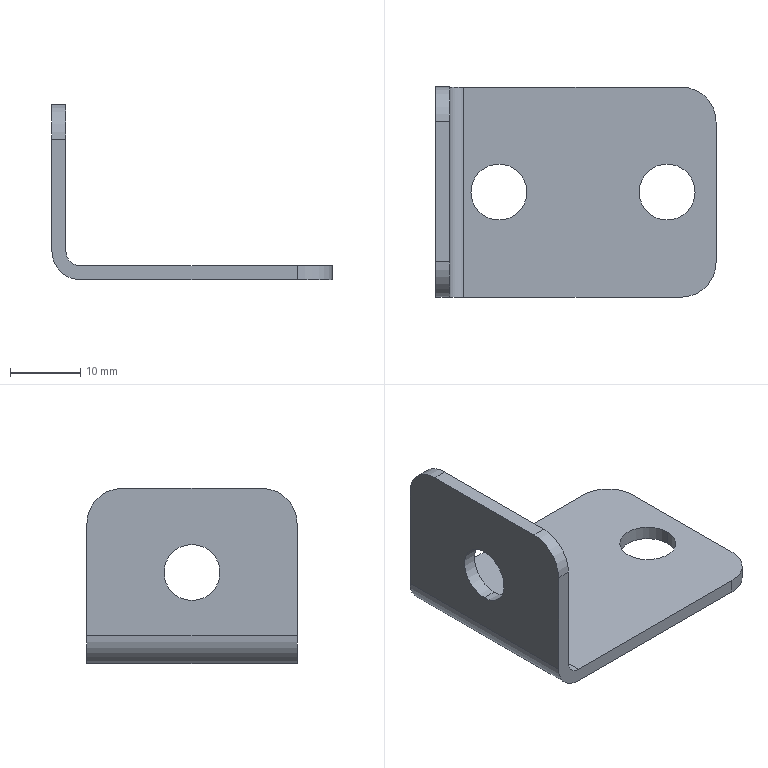Part | STEP file | 921271505 | 1 solid | 20 faces | box 40 x 30 x 25 mm | volume 3358 mm3 | cylinder 12 | plane 8 | commonest cylinder face diameters 8 x7 10 x4 4 x1
STEP:
#1=CARTESIAN_POINT('',(5.,15.,2.));
#2=VERTEX_POINT('',#1);
#3=CARTESIAN_POINT('',(13.,15.,2.));
#4=VERTEX_POINT('',#3);
#5=CARTESIAN_POINT('',(9.,15.,2.));
#6=DIRECTION('',(0.,0.,1.));
#7=DIRECTION('',(-1.,0.,0.));
#8=AXIS2_PLACEMENT_3D('',#5,#6,#7);
#9=CIRCLE('',#8,4.);
#10=EDGE_CURVE('',#2,#4,#9,.T.);
#11=ORIENTED_EDGE('',*,*,#10,.T.);
#12=CARTESIAN_POINT('',(13.,15.,0.));
#13=VERTEX_POINT('',#12);
#14=CARTESIAN_POINT('',(13.,15.,55.902));
#15=DIRECTION('',(0.,0.,-1.));
#16=VECTOR('',#15,1000.);
#17=LINE('',#14,#16);
#18=EDGE_CURVE('',#4,#13,#17,.T.);
#19=ORIENTED_EDGE('',*,*,#18,.T.);
#20=CARTESIAN_POINT('',(5.,15.,0.));
#21=VERTEX_POINT('',#20);
#22=CARTESIAN_POINT('',(9.,15.,0.));
#23=DIRECTION('',(0.,0.,1.));
#24=DIRECTION('',(-1.,0.,0.));
#25=AXIS2_PLACEMENT_3D('',#22,#23,#24);
#26=CIRCLE('',#25,4.);
#27=EDGE_CURVE('',#21,#13,#26,.T.);
#28=ORIENTED_EDGE('',*,*,#27,.F.);
#29=CARTESIAN_POINT('',(5.,15.,55.902));
#30=DIRECTION('',(0.,0.,-1.));
#31=VECTOR('',#30,1000.);
#32=LINE('',#29,#31);
#33=EDGE_CURVE('',#2,#21,#32,.T.);
#34=ORIENTED_EDGE('',*,*,#33,.F.);
#35=EDGE_LOOP('',(#11,#19,#28,#34));
#36=FACE_OUTER_BOUND('',#35,.T.);
#37=CARTESIAN_POINT('',(9.,15.,55.902));
#38=DIRECTION('',(0.,0.,-1.));
#39=DIRECTION('',(-1.,0.,0.));
#40=AXIS2_PLACEMENT_3D('',#37,#38,#39);
#41=CYLINDRICAL_SURFACE('',#40,4.);
#42=ADVANCED_FACE('',(#36),#41,.F.);
#43=CARTESIAN_POINT('',(29.,15.,2.));
#44=VERTEX_POINT('',#43);
#45=CARTESIAN_POINT('',(37.,15.,2.));
#46=VERTEX_POINT('',#45);
#47=CARTESIAN_POINT('',(33.,15.,2.));
#48=DIRECTION('',(0.,0.,1.));
#49=DIRECTION('',(-1.,0.,0.));
#50=AXIS2_PLACEMENT_3D('',#47,#48,#49);
#51=CIRCLE('',#50,4.);
#52=EDGE_CURVE('',#44,#46,#51,.T.);
#53=ORIENTED_EDGE('',*,*,#52,.T.);
#54=CARTESIAN_POINT('',(37.,15.,0.));
#55=VERTEX_POINT('',#54);
#56=CARTESIAN_POINT('',(37.,15.,55.902));
#57=DIRECTION('',(0.,0.,-1.));
#58=VECTOR('',#57,1000.);
#59=LINE('',#56,#58);
#60=EDGE_CURVE('',#46,#55,#59,.T.);
#61=ORIENTED_EDGE('',*,*,#60,.T.);
#62=CARTESIAN_POINT('',(29.,15.,0.));
#63=VERTEX_POINT('',#62);
#64=CARTESIAN_POINT('',(33.,15.,0.));
#65=DIRECTION('',(0.,0.,1.));
#66=DIRECTION('',(-1.,0.,0.));
#67=AXIS2_PLACEMENT_3D('',#64,#65,#66);
#68=CIRCLE('',#67,4.);
#69=EDGE_CURVE('',#63,#55,#68,.T.);
#70=ORIENTED_EDGE('',*,*,#69,.F.);
#71=CARTESIAN_POINT('',(29.,15.,55.902));
#72=DIRECTION('',(0.,0.,-1.));
#73=VECTOR('',#72,1000.);
#74=LINE('',#71,#73);
#75=EDGE_CURVE('',#44,#63,#74,.T.);
#76=ORIENTED_EDGE('',*,*,#75,.F.);
#77=EDGE_LOOP('',(#53,#61,#70,#76));
#78=FACE_OUTER_BOUND('',#77,.T.);
#79=CARTESIAN_POINT('',(33.,15.,55.902));
#80=DIRECTION('',(0.,0.,-1.));
#81=DIRECTION('',(-1.,0.,0.));
#82=AXIS2_PLACEMENT_3D('',#79,#80,#81);
#83=CYLINDRICAL_SURFACE('',#82,4.);
#84=ADVANCED_FACE('',(#78),#83,.F.);
#85=CARTESIAN_POINT('',(2.,15.,17.));
#86=VERTEX_POINT('',#85);
#87=CARTESIAN_POINT('',(2.,15.,9.));
#88=VERTEX_POINT('',#87);
#89=CARTESIAN_POINT('',(2.,15.,13.));
#90=DIRECTION('',(1.,0.,0.));
#91=DIRECTION('',(0.,0.,1.));
#92=AXIS2_PLACEMENT_3D('',#89,#90,#91);
#93=CIRCLE('',#92,4.);
#94=EDGE_CURVE('',#86,#88,#93,.T.);
#95=ORIENTED_EDGE('',*,*,#94,.T.);
#96=CARTESIAN_POINT('',(0.,15.,9.));
#97=VERTEX_POINT('',#96);
#98=CARTESIAN_POINT('',(55.902,15.,9.));
#99=DIRECTION('',(-1.,0.,0.));
#100=VECTOR('',#99,1000.);
#101=LINE('',#98,#100);
#102=EDGE_CURVE('',#88,#97,#101,.T.);
#103=ORIENTED_EDGE('',*,*,#102,.T.);
#104=CARTESIAN_POINT('',(0.,15.,17.));
#105=VERTEX_POINT('',#104);
#106=CARTESIAN_POINT('',(0.,15.,13.));
#107=DIRECTION('',(1.,0.,0.));
#108=DIRECTION('',(0.,0.,1.));
#109=AXIS2_PLACEMENT_3D('',#106,#107,#108);
#110=CIRCLE('',#109,4.);
#111=EDGE_CURVE('',#105,#97,#110,.T.);
#112=ORIENTED_EDGE('',*,*,#111,.F.);
#113=CARTESIAN_POINT('',(55.902,15.,17.));
#114=DIRECTION('',(-1.,0.,0.));
#115=VECTOR('',#114,1000.);
#116=LINE('',#113,#115);
#117=EDGE_CURVE('',#86,#105,#116,.T.);
#118=ORIENTED_EDGE('',*,*,#117,.F.);
#119=EDGE_LOOP('',(#95,#103,#112,#118));
#120=FACE_OUTER_BOUND('',#119,.T.);
#121=CARTESIAN_POINT('',(55.902,15.,13.));
#122=DIRECTION('',(-1.,0.,0.));
#123=DIRECTION('',(0.,0.,1.));
#124=AXIS2_PLACEMENT_3D('',#121,#122,#123);
#125=CYLINDRICAL_SURFACE('',#124,4.);
#126=ADVANCED_FACE('',(#120),#125,.F.);
#127=CARTESIAN_POINT('',(35.,30.,2.));
#128=VERTEX_POINT('',#127);
#129=CARTESIAN_POINT('',(40.,25.,2.));
#130=VERTEX_POINT('',#129);
#131=CARTESIAN_POINT('',(35.,25.,2.));
#132=DIRECTION('',(0.,0.,-1.));
#133=DIRECTION('',(-1.,0.,0.));
#134=AXIS2_PLACEMENT_3D('',#131,#132,#133);
#135=CIRCLE('',#134,5.);
#136=EDGE_CURVE('',#128,#130,#135,.T.);
#137=ORIENTED_EDGE('',*,*,#136,.F.);
#138=CARTESIAN_POINT('',(4.,30.,2.));
#139=VERTEX_POINT('',#138);
#140=CARTESIAN_POINT('',(0.,30.,2.));
#141=DIRECTION('',(1.,0.,0.));
#142=VECTOR('',#141,1000.);
#143=LINE('',#140,#142);
#144=EDGE_CURVE('',#139,#128,#143,.T.);
#145=ORIENTED_EDGE('',*,*,#144,.F.);
#146=CARTESIAN_POINT('',(4.,0.,2.));
#147=VERTEX_POINT('',#146);
#148=CARTESIAN_POINT('',(4.,0.,2.));
#149=DIRECTION('',(0.,1.,0.));
#150=VECTOR('',#149,1000.);
#151=LINE('',#148,#150);
#152=EDGE_CURVE('',#147,#139,#151,.T.);
#153=ORIENTED_EDGE('',*,*,#152,.F.);
#154=CARTESIAN_POINT('',(35.,0.,2.));
#155=VERTEX_POINT('',#154);
#156=CARTESIAN_POINT('',(0.,0.,2.));
#157=DIRECTION('',(-1.,0.,0.));
#158=VECTOR('',#157,1000.);
#159=LINE('',#156,#158);
#160=EDGE_CURVE('',#155,#147,#159,.T.);
#161=ORIENTED_EDGE('',*,*,#160,.F.);
#162=CARTESIAN_POINT('',(40.,5.,2.));
#163=VERTEX_POINT('',#162);
#164=CARTESIAN_POINT('',(35.,5.,2.));
#165=DIRECTION('',(0.,0.,-1.));
#166=DIRECTION('',(-1.,0.,0.));
#167=AXIS2_PLACEMENT_3D('',#164,#165,#166);
#168=CIRCLE('',#167,5.);
#169=EDGE_CURVE('',#163,#155,#168,.T.);
#170=ORIENTED_EDGE('',*,*,#169,.F.);
#171=CARTESIAN_POINT('',(40.,0.,2.));
#172=DIRECTION('',(0.,-1.,0.));
#173=VECTOR('',#172,1000.);
#174=LINE('',#171,#173);
#175=EDGE_CURVE('',#130,#163,#174,.T.);
#176=ORIENTED_EDGE('',*,*,#175,.F.);
#177=EDGE_LOOP('',(#137,#145,#153,#161,#170,#176));
#178=FACE_OUTER_BOUND('',#177,.T.);
#179=ORIENTED_EDGE('',*,*,#10,.F.);
#180=CARTESIAN_POINT('',(9.,15.,2.));
#181=DIRECTION('',(0.,0.,1.));
#182=DIRECTION('',(-1.,0.,0.));
#183=AXIS2_PLACEMENT_3D('',#180,#181,#182);
#184=CIRCLE('',#183,4.);
#185=EDGE_CURVE('',#4,#2,#184,.T.);
#186=ORIENTED_EDGE('',*,*,#185,.F.);
#187=EDGE_LOOP('',(#179,#186));
#188=FACE_BOUND('',#187,.T.);
#189=ORIENTED_EDGE('',*,*,#52,.F.);
#190=CARTESIAN_POINT('',(33.,15.,2.));
#191=DIRECTION('',(0.,0.,1.));
#192=DIRECTION('',(-1.,0.,0.));
#193=AXIS2_PLACEMENT_3D('',#190,#191,#192);
#194=CIRCLE('',#193,4.);
#195=EDGE_CURVE('',#46,#44,#194,.T.);
#196=ORIENTED_EDGE('',*,*,#195,.F.);
#197=EDGE_LOOP('',(#189,#196));
#198=FACE_BOUND('',#197,.T.);
#199=CARTESIAN_POINT('',(0.,0.,2.));
#200=DIRECTION('',(0.,0.,-1.));
#201=DIRECTION('',(-1.,0.,0.));
#202=AXIS2_PLACEMENT_3D('',#199,#200,#201);
#203=PLANE('',#202);
#204=ADVANCED_FACE('',(#178,#188,#198),#203,.F.);
#205=ORIENTED_EDGE('',*,*,#175,.T.);
#206=CARTESIAN_POINT('',(40.,5.,0.));
#207=VERTEX_POINT('',#206);
#208=CARTESIAN_POINT('',(40.,5.,2.));
#209=DIRECTION('',(0.,0.,-1.));
#210=VECTOR('',#209,1000.);
#211=LINE('',#208,#210);
#212=EDGE_CURVE('',#163,#207,#211,.T.);
#213=ORIENTED_EDGE('',*,*,#212,.T.);
#214=CARTESIAN_POINT('',(40.,25.,0.));
#215=VERTEX_POINT('',#214);
#216=CARTESIAN_POINT('',(40.,30.,0.));
#217=DIRECTION('',(0.,1.,0.));
#218=VECTOR('',#217,1000.);
#219=LINE('',#216,#218);
#220=EDGE_CURVE('',#207,#215,#219,.T.);
#221=ORIENTED_EDGE('',*,*,#220,.T.);
#222=CARTESIAN_POINT('',(40.,25.,2.));
#223=DIRECTION('',(0.,0.,1.));
#224=VECTOR('',#223,1000.);
#225=LINE('',#222,#224);
#226=EDGE_CURVE('',#215,#130,#225,.T.);
#227=ORIENTED_EDGE('',*,*,#226,.T.);
#228=EDGE_LOOP('',(#205,#213,#221,#227));
#229=FACE_OUTER_BOUND('',#228,.T.);
#230=CARTESIAN_POINT('',(40.,30.,2.));
#231=DIRECTION('',(1.,0.,0.));
#232=DIRECTION('',(0.,1.,0.));
#233=AXIS2_PLACEMENT_3D('',#230,#231,#232);
#234=PLANE('',#233);
#235=ADVANCED_FACE('',(#229),#234,.T.);
#236=CARTESIAN_POINT('',(35.,30.,0.));
#237=VERTEX_POINT('',#236);
#238=CARTESIAN_POINT('',(35.,25.,0.));
#239=DIRECTION('',(0.,0.,1.));
#240=DIRECTION('',(-1.,0.,0.));
#241=AXIS2_PLACEMENT_3D('',#238,#239,#240);
#242=CIRCLE('',#241,5.);
#243=EDGE_CURVE('',#215,#237,#242,.T.);
#244=ORIENTED_EDGE('',*,*,#243,.T.);
#245=CARTESIAN_POINT('',(35.,30.,2.));
#246=DIRECTION('',(0.,0.,1.));
#247=VECTOR('',#246,1000.);
#248=LINE('',#245,#247);
#249=EDGE_CURVE('',#237,#128,#248,.T.);
#250=ORIENTED_EDGE('',*,*,#249,.T.);
#251=ORIENTED_EDGE('',*,*,#136,.T.);
#252=ORIENTED_EDGE('',*,*,#226,.F.);
#253=EDGE_LOOP('',(#244,#250,#251,#252));
#254=FACE_OUTER_BOUND('',#253,.T.);
#255=CARTESIAN_POINT('',(35.,25.,2.));
#256=DIRECTION('',(0.,0.,-1.));
#257=DIRECTION('',(-1.,0.,0.));
#258=AXIS2_PLACEMENT_3D('',#255,#256,#257);
#259=CYLINDRICAL_SURFACE('',#258,5.);
#260=ADVANCED_FACE('',(#254),#259,.T.);
#261=CARTESIAN_POINT('',(4.,30.,0.));
#262=VERTEX_POINT('',#261);
#263=CARTESIAN_POINT('',(0.,30.,0.));
#264=DIRECTION('',(-1.,0.,0.));
#265=VECTOR('',#264,1000.);
#266=LINE('',#263,#265);
#267=EDGE_CURVE('',#237,#262,#266,.T.);
#268=ORIENTED_EDGE('',*,*,#267,.T.);
#269=CARTESIAN_POINT('',(0.,30.,4.));
#270=VERTEX_POINT('',#269);
#271=CARTESIAN_POINT('',(4.,30.,4.));
#272=DIRECTION('',(0.,1.,0.));
#273=DIRECTION('',(-1.,0.,0.));
#274=AXIS2_PLACEMENT_3D('',#271,#272,#273);
#275=CIRCLE('',#274,4.);
#276=EDGE_CURVE('',#262,#270,#275,.T.);
#277=ORIENTED_EDGE('',*,*,#276,.T.);
#278=CARTESIAN_POINT('',(0.,30.,20.));
#279=VERTEX_POINT('',#278);
#280=CARTESIAN_POINT('',(0.,30.,2.));
#281=DIRECTION('',(0.,0.,1.));
#282=VECTOR('',#281,1000.);
#283=LINE('',#280,#282);
#284=EDGE_CURVE('',#270,#279,#283,.T.);
#285=ORIENTED_EDGE('',*,*,#284,.T.);
#286=CARTESIAN_POINT('',(2.,30.,20.));
#287=VERTEX_POINT('',#286);
#288=CARTESIAN_POINT('',(0.,30.,20.));
#289=DIRECTION('',(1.,0.,0.));
#290=VECTOR('',#289,1000.);
#291=LINE('',#288,#290);
#292=EDGE_CURVE('',#279,#287,#291,.T.);
#293=ORIENTED_EDGE('',*,*,#292,.T.);
#294=CARTESIAN_POINT('',(2.,30.,4.));
#295=VERTEX_POINT('',#294);
#296=CARTESIAN_POINT('',(2.,30.,2.));
#297=DIRECTION('',(0.,0.,-1.));
#298=VECTOR('',#297,1000.);
#299=LINE('',#296,#298);
#300=EDGE_CURVE('',#287,#295,#299,.T.);
#301=ORIENTED_EDGE('',*,*,#300,.T.);
#302=CARTESIAN_POINT('',(4.,30.,4.));
#303=DIRECTION('',(0.,-1.,0.));
#304=DIRECTION('',(-1.,0.,0.));
#305=AXIS2_PLACEMENT_3D('',#302,#303,#304);
#306=CIRCLE('',#305,2.);
#307=EDGE_CURVE('',#295,#139,#306,.T.);
#308=ORIENTED_EDGE('',*,*,#307,.T.);
#309=ORIENTED_EDGE('',*,*,#144,.T.);
#310=ORIENTED_EDGE('',*,*,#249,.F.);
#311=EDGE_LOOP('',(#268,#277,#285,#293,#301,#308,#309,#310));
#312=FACE_OUTER_BOUND('',#311,.T.);
#313=CARTESIAN_POINT('',(0.,30.,2.));
#314=DIRECTION('',(0.,1.,0.));
#315=DIRECTION('',(0.,0.,1.));
#316=AXIS2_PLACEMENT_3D('',#313,#314,#315);
#317=PLANE('',#316);
#318=ADVANCED_FACE('',(#312),#317,.T.);
#319=ORIENTED_EDGE('',*,*,#307,.F.);
#320=CARTESIAN_POINT('',(2.,0.,4.));
#321=VERTEX_POINT('',#320);
#322=CARTESIAN_POINT('',(2.,0.,4.));
#323=DIRECTION('',(0.,1.,0.));
#324=VECTOR('',#323,1000.);
#325=LINE('',#322,#324);
#326=EDGE_CURVE('',#321,#295,#325,.T.);
#327=ORIENTED_EDGE('',*,*,#326,.F.);
#328=CARTESIAN_POINT('',(4.,0.,4.));
#329=DIRECTION('',(0.,1.,0.));
#330=DIRECTION('',(-1.,0.,0.));
#331=AXIS2_PLACEMENT_3D('',#328,#329,#330);
#332=CIRCLE('',#331,2.);
#333=EDGE_CURVE('',#147,#321,#332,.T.);
#334=ORIENTED_EDGE('',*,*,#333,.F.);
#335=ORIENTED_EDGE('',*,*,#152,.T.);
#336=EDGE_LOOP('',(#319,#327,#334,#335));
#337=FACE_OUTER_BOUND('',#336,.T.);
#338=CARTESIAN_POINT('',(4.,0.,4.));
#339=DIRECTION('',(0.,1.,0.));
#340=DIRECTION('',(-1.,0.,0.));
#341=AXIS2_PLACEMENT_3D('',#338,#339,#340);
#342=CYLINDRICAL_SURFACE('',#341,2.);
#343=ADVANCED_FACE('',(#337),#342,.F.);
#344=ORIENTED_EDGE('',*,*,#160,.T.);
#345=ORIENTED_EDGE('',*,*,#333,.T.);
#346=CARTESIAN_POINT('',(2.,0.,20.));
#347=VERTEX_POINT('',#346);
#348=CARTESIAN_POINT('',(2.,0.,2.));
#349=DIRECTION('',(0.,0.,1.));
#350=VECTOR('',#349,1000.);
#351=LINE('',#348,#350);
#352=EDGE_CURVE('',#321,#347,#351,.T.);
#353=ORIENTED_EDGE('',*,*,#352,.T.);
#354=CARTESIAN_POINT('',(0.,0.,20.));
#355=VERTEX_POINT('',#354);
#356=CARTESIAN_POINT('',(40.,0.,20.));
#357=DIRECTION('',(-1.,0.,0.));
#358=VECTOR('',#357,1000.);
#359=LINE('',#356,#358);
#360=EDGE_CURVE('',#347,#355,#359,.T.);
#361=ORIENTED_EDGE('',*,*,#360,.T.);
#362=CARTESIAN_POINT('',(0.,0.,4.));
#363=VERTEX_POINT('',#362);
#364=CARTESIAN_POINT('',(0.,0.,2.));
#365=DIRECTION('',(0.,0.,-1.));
#366=VECTOR('',#365,1000.);
#367=LINE('',#364,#366);
#368=EDGE_CURVE('',#355,#363,#367,.T.);
#369=ORIENTED_EDGE('',*,*,#368,.T.);
#370=CARTESIAN_POINT('',(4.,0.,0.));
#371=VERTEX_POINT('',#370);
#372=CARTESIAN_POINT('',(4.,0.,4.));
#373=DIRECTION('',(0.,-1.,0.));
#374=DIRECTION('',(-1.,0.,0.));
#375=AXIS2_PLACEMENT_3D('',#372,#373,#374);
#376=CIRCLE('',#375,4.);
#377=EDGE_CURVE('',#363,#371,#376,.T.);
#378=ORIENTED_EDGE('',*,*,#377,.T.);
#379=CARTESIAN_POINT('',(35.,0.,0.));
#380=VERTEX_POINT('',#379);
#381=CARTESIAN_POINT('',(40.,0.,0.));
#382=DIRECTION('',(1.,0.,0.));
#383=VECTOR('',#382,1000.);
#384=LINE('',#381,#383);
#385=EDGE_CURVE('',#371,#380,#384,.T.);
#386=ORIENTED_EDGE('',*,*,#385,.T.);
#387=CARTESIAN_POINT('',(35.,0.,2.));
#388=DIRECTION('',(0.,0.,1.));
#389=VECTOR('',#388,1000.);
#390=LINE('',#387,#389);
#391=EDGE_CURVE('',#380,#155,#390,.T.);
#392=ORIENTED_EDGE('',*,*,#391,.T.);
#393=EDGE_LOOP('',(#344,#345,#353,#361,#369,#378,#386,#392));
#394=FACE_OUTER_BOUND('',#393,.T.);
#395=CARTESIAN_POINT('',(40.,0.,2.));
#396=DIRECTION('',(0.,-1.,0.));
#397=DIRECTION('',(0.,0.,-1.));
#398=AXIS2_PLACEMENT_3D('',#395,#396,#397);
#399=PLANE('',#398);
#400=ADVANCED_FACE('',(#394),#399,.T.);
#401=CARTESIAN_POINT('',(35.,5.,0.));
#402=DIRECTION('',(0.,0.,1.));
#403=DIRECTION('',(-1.,0.,0.));
#404=AXIS2_PLACEMENT_3D('',#401,#402,#403);
#405=CIRCLE('',#404,5.);
#406=EDGE_CURVE('',#380,#207,#405,.T.);
#407=ORIENTED_EDGE('',*,*,#406,.T.);
#408=ORIENTED_EDGE('',*,*,#212,.F.);
#409=ORIENTED_EDGE('',*,*,#169,.T.);
#410=ORIENTED_EDGE('',*,*,#391,.F.);
#411=EDGE_LOOP('',(#407,#408,#409,#410));
#412=FACE_OUTER_BOUND('',#411,.T.);
#413=CARTESIAN_POINT('',(35.,5.,2.));
#414=DIRECTION('',(0.,0.,-1.));
#415=DIRECTION('',(-1.,0.,0.));
#416=AXIS2_PLACEMENT_3D('',#413,#414,#415);
#417=CYLINDRICAL_SURFACE('',#416,5.);
#418=ADVANCED_FACE('',(#412),#417,.T.);
#419=ORIENTED_EDGE('',*,*,#18,.F.);
#420=ORIENTED_EDGE('',*,*,#185,.T.);
#421=ORIENTED_EDGE('',*,*,#33,.T.);
#422=CARTESIAN_POINT('',(9.,15.,0.));
#423=DIRECTION('',(0.,0.,1.));
#424=DIRECTION('',(-1.,0.,0.));
#425=AXIS2_PLACEMENT_3D('',#422,#423,#424);
#426=CIRCLE('',#425,4.);
#427=EDGE_CURVE('',#13,#21,#426,.T.);
#428=ORIENTED_EDGE('',*,*,#427,.F.);
#429=EDGE_LOOP('',(#419,#420,#421,#428));
#430=FACE_OUTER_BOUND('',#429,.T.);
#431=CARTESIAN_POINT('',(9.,15.,55.902));
#432=DIRECTION('',(0.,0.,-1.));
#433=DIRECTION('',(-1.,0.,0.));
#434=AXIS2_PLACEMENT_3D('',#431,#432,#433);
#435=CYLINDRICAL_SURFACE('',#434,4.);
#436=ADVANCED_FACE('',(#430),#435,.F.);
#437=ORIENTED_EDGE('',*,*,#60,.F.);
#438=ORIENTED_EDGE('',*,*,#195,.T.);
#439=ORIENTED_EDGE('',*,*,#75,.T.);
#440=CARTESIAN_POINT('',(33.,15.,0.));
#441=DIRECTION('',(0.,0.,1.));
#442=DIRECTION('',(-1.,0.,0.));
#443=AXIS2_PLACEMENT_3D('',#440,#441,#442);
#444=CIRCLE('',#443,4.);
#445=EDGE_CURVE('',#55,#63,#444,.T.);
#446=ORIENTED_EDGE('',*,*,#445,.F.);
#447=EDGE_LOOP('',(#437,#438,#439,#446));
#448=FACE_OUTER_BOUND('',#447,.T.);
#449=CARTESIAN_POINT('',(33.,15.,55.902));
#450=DIRECTION('',(0.,0.,-1.));
#451=DIRECTION('',(-1.,0.,0.));
#452=AXIS2_PLACEMENT_3D('',#449,#450,#451);
#453=CYLINDRICAL_SURFACE('',#452,4.);
#454=ADVANCED_FACE('',(#448),#453,.F.);
#455=ORIENTED_EDGE('',*,*,#385,.F.);
#456=CARTESIAN_POINT('',(4.,0.,0.));
#457=DIRECTION('',(0.,1.,0.));
#458=VECTOR('',#457,1000.);
#459=LINE('',#456,#458);
#460=EDGE_CURVE('',#371,#262,#459,.T.);
#461=ORIENTED_EDGE('',*,*,#460,.T.);
#462=ORIENTED_EDGE('',*,*,#267,.F.);
#463=ORIENTED_EDGE('',*,*,#243,.F.);
#464=ORIENTED_EDGE('',*,*,#220,.F.);
#465=ORIENTED_EDGE('',*,*,#406,.F.);
#466=EDGE_LOOP('',(#455,#461,#462,#463,#464,#465));
#467=FACE_OUTER_BOUND('',#466,.T.);
#468=ORIENTED_EDGE('',*,*,#27,.T.);
#469=ORIENTED_EDGE('',*,*,#427,.T.);
#470=EDGE_LOOP('',(#468,#469));
#471=FACE_BOUND('',#470,.T.);
#472=ORIENTED_EDGE('',*,*,#69,.T.);
#473=ORIENTED_EDGE('',*,*,#445,.T.);
#474=EDGE_LOOP('',(#472,#473));
#475=FACE_BOUND('',#474,.T.);
#476=CARTESIAN_POINT('',(0.,0.,0.));
#477=DIRECTION('',(0.,0.,-1.));
#478=DIRECTION('',(-1.,0.,0.));
#479=AXIS2_PLACEMENT_3D('',#476,#477,#478);
#480=PLANE('',#479);
#481=ADVANCED_FACE('',(#467,#471,#475),#480,.T.);
#482=CARTESIAN_POINT('',(0.,0.,4.));
#483=DIRECTION('',(0.,1.,0.));
#484=VECTOR('',#483,1000.);
#485=LINE('',#482,#484);
#486=EDGE_CURVE('',#363,#270,#485,.T.);
#487=ORIENTED_EDGE('',*,*,#486,.T.);
#488=ORIENTED_EDGE('',*,*,#276,.F.);
#489=ORIENTED_EDGE('',*,*,#460,.F.);
#490=ORIENTED_EDGE('',*,*,#377,.F.);
#491=EDGE_LOOP('',(#487,#488,#489,#490));
#492=FACE_OUTER_BOUND('',#491,.T.);
#493=CARTESIAN_POINT('',(4.,0.,4.));
#494=DIRECTION('',(0.,1.,0.));
#495=DIRECTION('',(-1.,0.,0.));
#496=AXIS2_PLACEMENT_3D('',#493,#494,#495);
#497=CYLINDRICAL_SURFACE('',#496,4.);
#498=ADVANCED_FACE('',(#492),#497,.T.);
#499=CARTESIAN_POINT('',(2.,5.,25.));
#500=VERTEX_POINT('',#499);
#501=CARTESIAN_POINT('',(2.,5.,20.));
#502=DIRECTION('',(-1.,0.,0.));
#503=DIRECTION('',(0.,0.,1.));
#504=AXIS2_PLACEMENT_3D('',#501,#502,#503);
#505=CIRCLE('',#504,5.);
#506=EDGE_CURVE('',#347,#500,#505,.T.);
#507=ORIENTED_EDGE('',*,*,#506,.F.);
#508=ORIENTED_EDGE('',*,*,#352,.F.);
#509=ORIENTED_EDGE('',*,*,#326,.T.);
#510=ORIENTED_EDGE('',*,*,#300,.F.);
#511=CARTESIAN_POINT('',(2.,25.,25.));
#512=VERTEX_POINT('',#511);
#513=CARTESIAN_POINT('',(2.,25.,20.));
#514=DIRECTION('',(-1.,0.,0.));
#515=DIRECTION('',(0.,0.,1.));
#516=AXIS2_PLACEMENT_3D('',#513,#514,#515);
#517=CIRCLE('',#516,5.);
#518=EDGE_CURVE('',#512,#287,#517,.T.);
#519=ORIENTED_EDGE('',*,*,#518,.F.);
#520=CARTESIAN_POINT('',(2.,0.,25.));
#521=DIRECTION('',(0.,1.,0.));
#522=VECTOR('',#521,1000.);
#523=LINE('',#520,#522);
#524=EDGE_CURVE('',#500,#512,#523,.T.);
#525=ORIENTED_EDGE('',*,*,#524,.F.);
#526=EDGE_LOOP('',(#507,#508,#509,#510,#519,#525));
#527=FACE_OUTER_BOUND('',#526,.T.);
#528=ORIENTED_EDGE('',*,*,#94,.F.);
#529=CARTESIAN_POINT('',(2.,15.,13.));
#530=DIRECTION('',(1.,0.,0.));
#531=DIRECTION('',(0.,0.,1.));
#532=AXIS2_PLACEMENT_3D('',#529,#530,#531);
#533=CIRCLE('',#532,4.);
#534=EDGE_CURVE('',#88,#86,#533,.T.);
#535=ORIENTED_EDGE('',*,*,#534,.F.);
#536=EDGE_LOOP('',(#528,#535));
#537=FACE_BOUND('',#536,.T.);
#538=CARTESIAN_POINT('',(2.,0.,0.));
#539=DIRECTION('',(-1.,0.,0.));
#540=DIRECTION('',(0.,0.,1.));
#541=AXIS2_PLACEMENT_3D('',#538,#539,#540);
#542=PLANE('',#541);
#543=ADVANCED_FACE('',(#527,#537),#542,.F.);
#544=ORIENTED_EDGE('',*,*,#518,.T.);
#545=ORIENTED_EDGE('',*,*,#292,.F.);
#546=CARTESIAN_POINT('',(0.,25.,25.));
#547=VERTEX_POINT('',#546);
#548=CARTESIAN_POINT('',(0.,25.,20.));
#549=DIRECTION('',(1.,0.,0.));
#550=DIRECTION('',(0.,0.,1.));
#551=AXIS2_PLACEMENT_3D('',#548,#549,#550);
#552=CIRCLE('',#551,5.);
#553=EDGE_CURVE('',#279,#547,#552,.T.);
#554=ORIENTED_EDGE('',*,*,#553,.T.);
#555=CARTESIAN_POINT('',(0.,25.,25.));
#556=DIRECTION('',(1.,0.,0.));
#557=VECTOR('',#556,1000.);
#558=LINE('',#555,#557);
#559=EDGE_CURVE('',#547,#512,#558,.T.);
#560=ORIENTED_EDGE('',*,*,#559,.T.);
#561=EDGE_LOOP('',(#544,#545,#554,#560));
#562=FACE_OUTER_BOUND('',#561,.T.);
#563=CARTESIAN_POINT('',(0.,25.,20.));
#564=DIRECTION('',(-1.,0.,0.));
#565=DIRECTION('',(0.,0.,1.));
#566=AXIS2_PLACEMENT_3D('',#563,#564,#565);
#567=CYLINDRICAL_SURFACE('',#566,5.);
#568=ADVANCED_FACE('',(#562),#567,.T.);
#569=ORIENTED_EDGE('',*,*,#284,.F.);
#570=ORIENTED_EDGE('',*,*,#486,.F.);
#571=ORIENTED_EDGE('',*,*,#368,.F.);
#572=CARTESIAN_POINT('',(0.,5.,25.));
#573=VERTEX_POINT('',#572);
#574=CARTESIAN_POINT('',(0.,5.,20.));
#575=DIRECTION('',(-1.,0.,0.));
#576=DIRECTION('',(0.,0.,1.));
#577=AXIS2_PLACEMENT_3D('',#574,#575,#576);
#578=CIRCLE('',#577,5.);
#579=EDGE_CURVE('',#355,#573,#578,.T.);
#580=ORIENTED_EDGE('',*,*,#579,.T.);
#581=CARTESIAN_POINT('',(0.,0.,25.));
#582=DIRECTION('',(0.,1.,0.));
#583=VECTOR('',#582,1000.);
#584=LINE('',#581,#583);
#585=EDGE_CURVE('',#573,#547,#584,.T.);
#586=ORIENTED_EDGE('',*,*,#585,.T.);
#587=ORIENTED_EDGE('',*,*,#553,.F.);
#588=EDGE_LOOP('',(#569,#570,#571,#580,#586,#587));
#589=FACE_OUTER_BOUND('',#588,.T.);
#590=ORIENTED_EDGE('',*,*,#111,.T.);
#591=CARTESIAN_POINT('',(0.,15.,13.));
#592=DIRECTION('',(1.,0.,0.));
#593=DIRECTION('',(0.,0.,1.));
#594=AXIS2_PLACEMENT_3D('',#591,#592,#593);
#595=CIRCLE('',#594,4.);
#596=EDGE_CURVE('',#97,#105,#595,.T.);
#597=ORIENTED_EDGE('',*,*,#596,.T.);
#598=EDGE_LOOP('',(#590,#597));
#599=FACE_BOUND('',#598,.T.);
#600=CARTESIAN_POINT('',(0.,0.,0.));
#601=DIRECTION('',(-1.,0.,0.));
#602=DIRECTION('',(0.,0.,1.));
#603=AXIS2_PLACEMENT_3D('',#600,#601,#602);
#604=PLANE('',#603);
#605=ADVANCED_FACE('',(#589,#599),#604,.T.);
#606=ORIENTED_EDGE('',*,*,#506,.T.);
#607=CARTESIAN_POINT('',(0.,5.,25.));
#608=DIRECTION('',(-1.,0.,0.));
#609=VECTOR('',#608,1000.);
#610=LINE('',#607,#609);
#611=EDGE_CURVE('',#500,#573,#610,.T.);
#612=ORIENTED_EDGE('',*,*,#611,.T.);
#613=ORIENTED_EDGE('',*,*,#579,.F.);
#614=ORIENTED_EDGE('',*,*,#360,.F.);
#615=EDGE_LOOP('',(#606,#612,#613,#614));
#616=FACE_OUTER_BOUND('',#615,.T.);
#617=CARTESIAN_POINT('',(0.,5.,20.));
#618=DIRECTION('',(-1.,0.,0.));
#619=DIRECTION('',(0.,0.,1.));
#620=AXIS2_PLACEMENT_3D('',#617,#618,#619);
#621=CYLINDRICAL_SURFACE('',#620,5.);
#622=ADVANCED_FACE('',(#616),#621,.T.);
#623=ORIENTED_EDGE('',*,*,#611,.F.);
#624=ORIENTED_EDGE('',*,*,#524,.T.);
#625=ORIENTED_EDGE('',*,*,#559,.F.);
#626=ORIENTED_EDGE('',*,*,#585,.F.);
#627=EDGE_LOOP('',(#623,#624,#625,#626));
#628=FACE_OUTER_BOUND('',#627,.T.);
#629=CARTESIAN_POINT('',(0.,0.,25.));
#630=DIRECTION('',(0.,0.,-1.));
#631=DIRECTION('',(-1.,0.,0.));
#632=AXIS2_PLACEMENT_3D('',#629,#630,#631);
#633=PLANE('',#632);
#634=ADVANCED_FACE('',(#628),#633,.F.);
#635=ORIENTED_EDGE('',*,*,#102,.F.);
#636=ORIENTED_EDGE('',*,*,#534,.T.);
#637=ORIENTED_EDGE('',*,*,#117,.T.);
#638=ORIENTED_EDGE('',*,*,#596,.F.);
#639=EDGE_LOOP('',(#635,#636,#637,#638));
#640=FACE_OUTER_BOUND('',#639,.T.);
#641=CARTESIAN_POINT('',(55.902,15.,13.));
#642=DIRECTION('',(-1.,0.,0.));
#643=DIRECTION('',(0.,0.,1.));
#644=AXIS2_PLACEMENT_3D('',#641,#642,#643);
#645=CYLINDRICAL_SURFACE('',#644,4.);
#646=ADVANCED_FACE('',(#640),#645,.F.);
#647=CLOSED_SHELL('',(#42,#84,#126,#204,#235,#260,#318,#343,#400,#418,#436,#454,#481,#498,#543,#568,#605,#622,#634,#646));
#648=MANIFOLD_SOLID_BREP('',#647);
#649=CARTESIAN_POINT('',(0.,0.,0.));
#650=DIRECTION('',(0.,0.,1.));
#651=DIRECTION('',(1.,0.,0.));
#652=AXIS2_PLACEMENT_3D('',#649,#650,#651);
#653=(LENGTH_UNIT()NAMED_UNIT(*)SI_UNIT(.MILLI.,.METRE.));
#654=UNCERTAINTY_MEASURE_WITH_UNIT(LENGTH_MEASURE(0.00001),#653,'','');
#655=(NAMED_UNIT(*)PLANE_ANGLE_UNIT()SI_UNIT($,.RADIAN.));
#656=(NAMED_UNIT(*)SI_UNIT($,.STERADIAN.)SOLID_ANGLE_UNIT());
#657=(GEOMETRIC_REPRESENTATION_CONTEXT(3)GLOBAL_UNCERTAINTY_ASSIGNED_CONTEXT((#654))GLOBAL_UNIT_ASSIGNED_CONTEXT((#653,#655,#656))REPRESENTATION_CONTEXT('',''));
#658=ADVANCED_BREP_SHAPE_REPRESENTATION('',(#648,#652),#657);